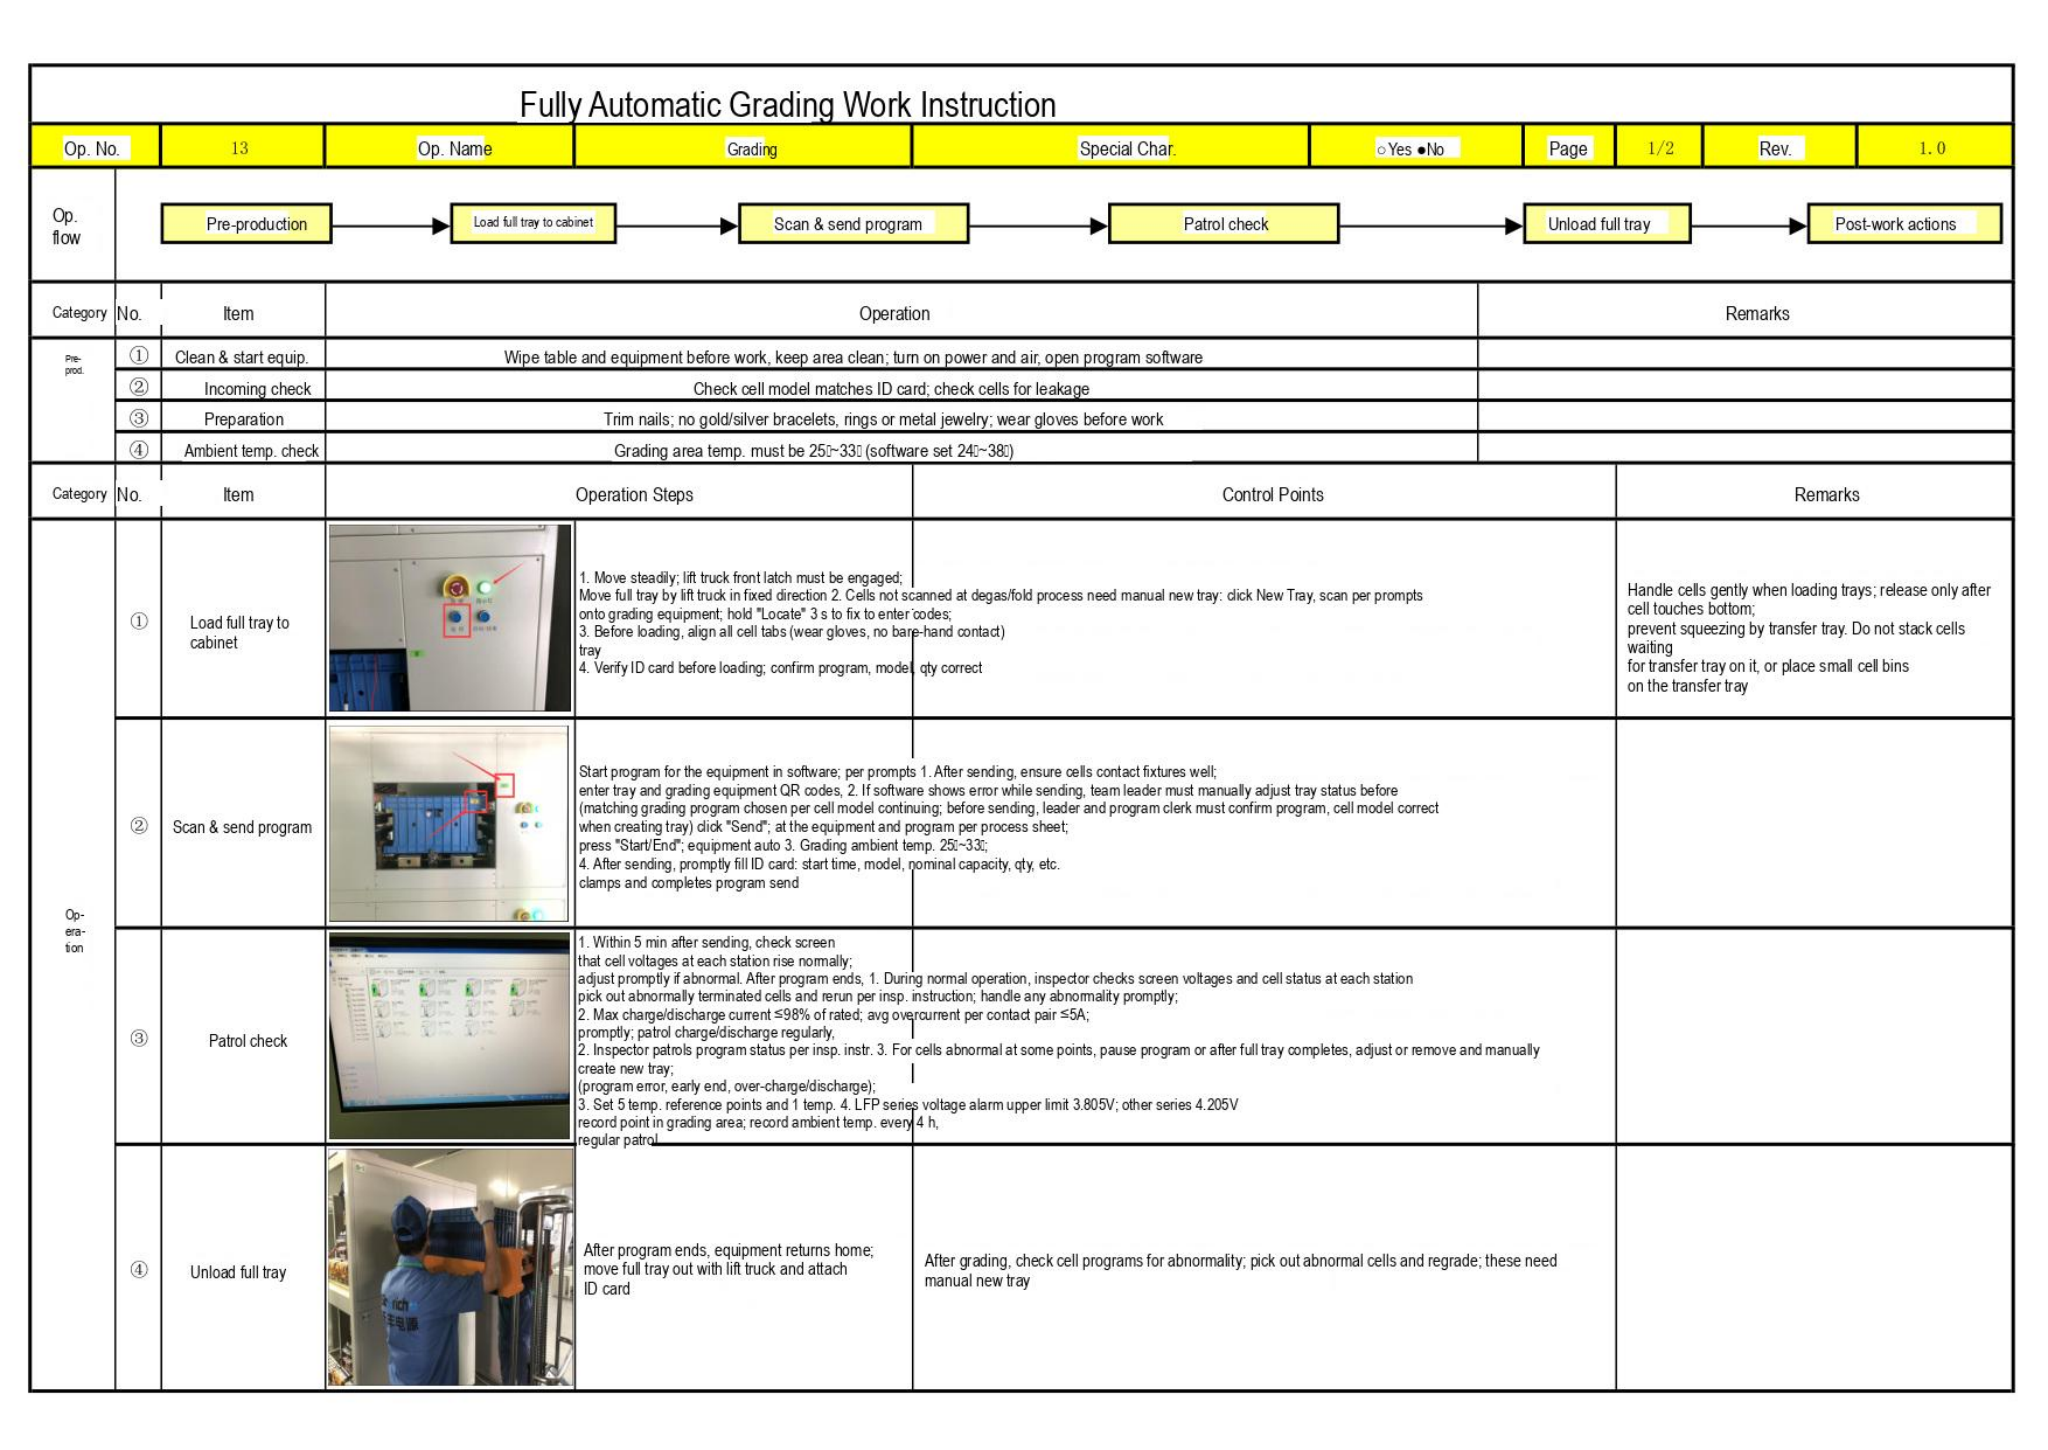# Fully Automatic Grading Work Instruction

| Op. No. | 13 | Op. Name | Grading | Special Char. | ○Yes ●No | Page | 1/2 | Rev. | 1.0 |
|---|---|---|---|---|---|---|---|---|---|

Op. flow: Pre-production → Load full tray to cabinet → Scan & send program → Patrol check → Unload full tray → Post-work actions

| Category | No. | Item | Operation | Remarks |
|---|---|---|---|---|
| Pre-prod. | ① | Clean & start equip. | Wipe table and equipment before work, keep area clean; turn on power and air, open program software | |
| | ② | Incoming check | Check cell model matches ID card; check cells for leakage | |
| | ③ | Preparation | Trim nails; no gold/silver bracelets, rings or metal jewelry; wear gloves before work | |
| | ④ | Ambient temp. check | Grading area temp. must be 25~33 (software set 24~38) | |

| Category | No. | Item | Operation Steps | Control Points | Remarks |
|---|---|---|---|---|---|
| Op-era-tion | ① | Load full tray to cabinet | 1. Move steadily; lift truck front latch must be engaged;<br>Move full tray by lift truck in fixed direction 2. Cells not scanned at degas/fold process need manual new tray: click New Tray, scan per prompts<br>onto grading equipment; hold "Locate" 3 s to fix to enter codes;<br>3. Before loading, align all cell tabs (wear gloves, no bare-hand contact)<br>tray<br>4. Verify ID card before loading; confirm program, model, qty correct | | Handle cells gently when loading trays; release only after cell touches bottom;<br>prevent squeezing by transfer tray. Do not stack cells waiting<br>for transfer tray on it, or place small cell bins<br>on the transfer tray |
| | ② | Scan & send program | Start program for the equipment in software; per prompts 1. After sending, ensure cells contact fixtures well;<br>enter tray and grading equipment QR codes, 2. If software shows error while sending, team leader must manually adjust tray status before<br>(matching grading program chosen per cell model continuing; before sending, leader and program clerk must confirm program, cell model correct<br>when creating tray) click "Send"; at the equipment and program per process sheet;<br>press "Start/End"; equipment auto 3. Grading ambient temp. 25~33;<br>4. After sending, promptly fill ID card: start time, model, nominal capacity, qty, etc.<br>clamps and completes program send | | |
| | ③ | Patrol check | 1. Within 5 min after sending, check screen<br>that cell voltages at each station rise normally;<br>adjust promptly if abnormal. After program ends, 1. During normal operation, inspector checks screen voltages and cell status at each station<br>pick out abnormally terminated cells and rerun per insp. instruction; handle any abnormality promptly;<br>2. Max charge/discharge current ≤98% of rated; avg overcurrent per contact pair ≤5A;<br>promptly; patrol charge/discharge regularly,<br>2. Inspector patrols program status per insp. instr. 3. For cells abnormal at some points, pause program or after full tray completes, adjust or remove and manually<br>create new tray;<br>(program error, early end, over-charge/discharge);<br>3. Set 5 temp. reference points and 1 temp. 4. LFP series voltage alarm upper limit 3.805V; other series 4.205V<br>record point in grading area; record ambient temp. every 4 h,<br>regular patrol | | |
| | ④ | Unload full tray | After program ends, equipment returns home; move full tray out with lift truck and attach ID card | After grading, check cell programs for abnormality; pick out abnormal cells and regrade; these need manual new tray | |
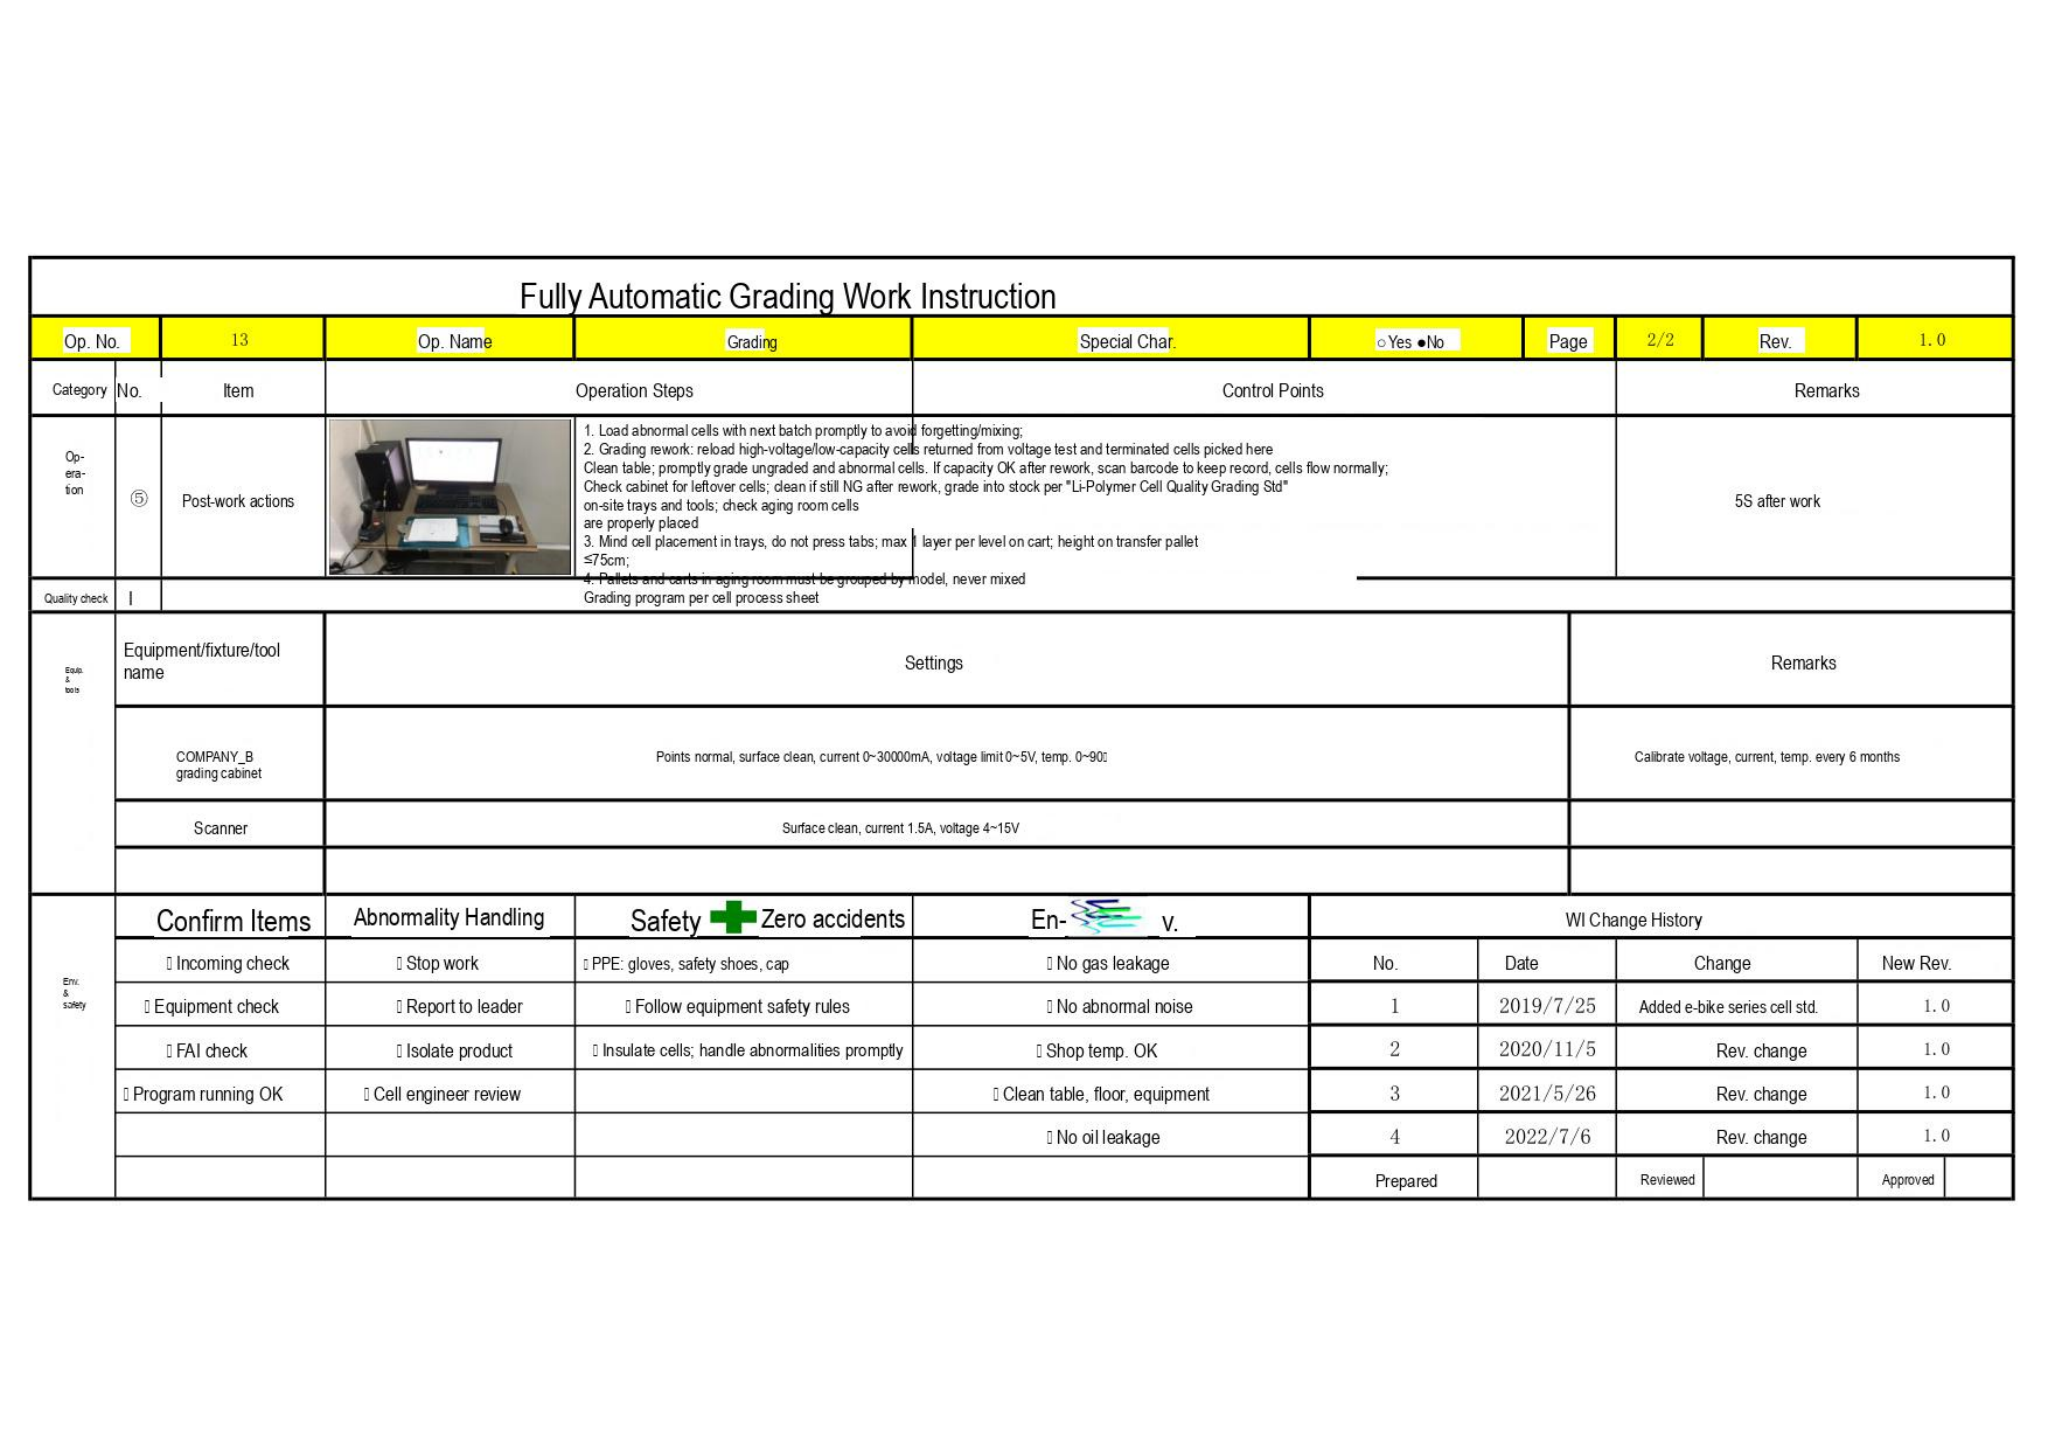# Fully Automatic Grading Work Instruction

| Op. No. | 13 | Op. Name | Grading | Special Char. | ○Yes ●No | Page | 2/2 | Rev. | 1.0 |
|---|---|---|---|---|---|---|---|---|---|

| Category | No. | Item | Operation Steps | Control Points | Remarks |
|---|---|---|---|---|---|
| Op-era-tion | ⑤ | Post-work actions | 1. Load abnormal cells with next batch promptly to avoid forgetting/mixing;<br>2. Grading rework: reload high-voltage/low-capacity cells returned from voltage test and terminated cells picked here<br>Clean table; promptly grade ungraded and abnormal cells. If capacity OK after rework, scan barcode to keep record, cells flow normally;<br>Check cabinet for leftover cells; clean if still NG after rework, grade into stock per "Li-Polymer Cell Quality Grading Std"<br>on-site trays and tools; check aging room cells<br>are properly placed<br>3. Mind cell placement in trays, do not press tabs; max 1 layer per level on cart; height on transfer pallet ≤75cm;<br>4. Pallets and carts in aging room must be grouped by model, never mixed | | 5S after work |
| Quality check | I | | Grading program per cell process sheet | | |

| Equip. & tools | Equipment/fixture/tool name | Settings | Remarks |
|---|---|---|---|
| | COMPANY_B grading cabinet | Points normal, surface clean, current 0~30000mA, voltage limit 0~5V, temp. 0~90 | Calibrate voltage, current, temp. every 6 months |
| | Scanner | Surface clean, current 1.5A, voltage 4~15V | |
| | | | |

| Env. & safety | Confirm Items | Abnormality Handling | Safety Zero accidents | En- v. | WI Change History | | | |
|---|---|---|---|---|---|---|---|---|
| | | | | | No. | Date | Change | New Rev. |
| | ▯ Incoming check | ▯ Stop work | ▯ PPE: gloves, safety shoes, cap | ▯ No gas leakage | 1 | 2019/7/25 | Added e-bike series cell std. | 1.0 |
| | ▯ Equipment check | ▯ Report to leader | ▯ Follow equipment safety rules | ▯ No abnormal noise | 2 | 2020/11/5 | Rev. change | 1.0 |
| | ▯ FAI check | ▯ Isolate product | ▯ Insulate cells; handle abnormalities promptly | ▯ Shop temp. OK | 3 | 2021/5/26 | Rev. change | 1.0 |
| | ▯ Program running OK | ▯ Cell engineer review | | ▯ Clean table, floor, equipment | 4 | 2022/7/6 | Rev. change | 1.0 |
| | | | | ▯ No oil leakage | Prepared | | Reviewed | Approved |